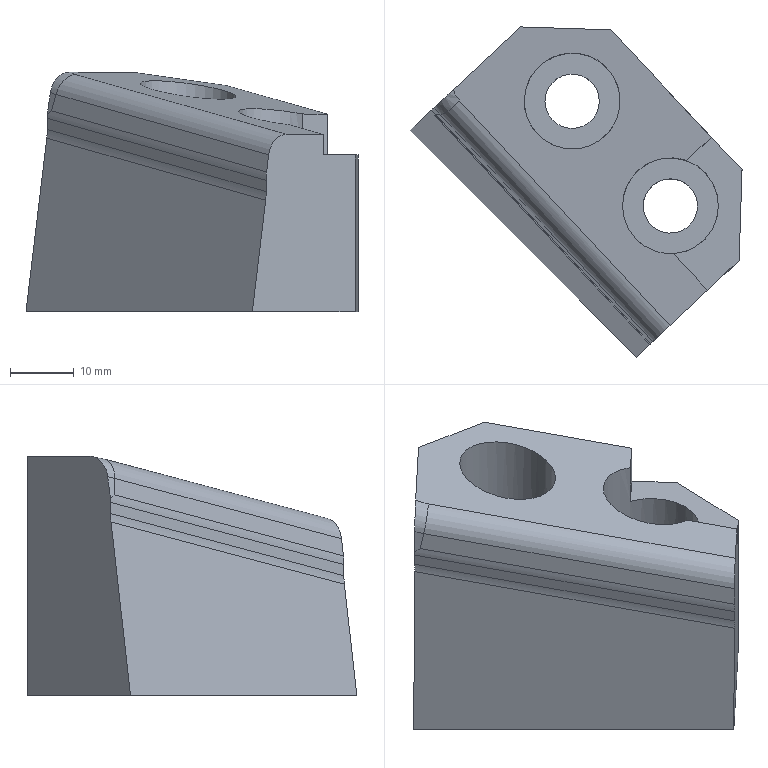Part | STEP file | gslz 2016.10.28-13_id102_x_t | 1 solid | 24 faces | box 51.891 x 51.539 x 37.446 mm | volume 37300 mm3 | plane 14 | cylinder 8 | spline 2 | commonest cylinder face diameters 8.5 x2 15 x2 16 x2 7.5 x1 17.5 x1